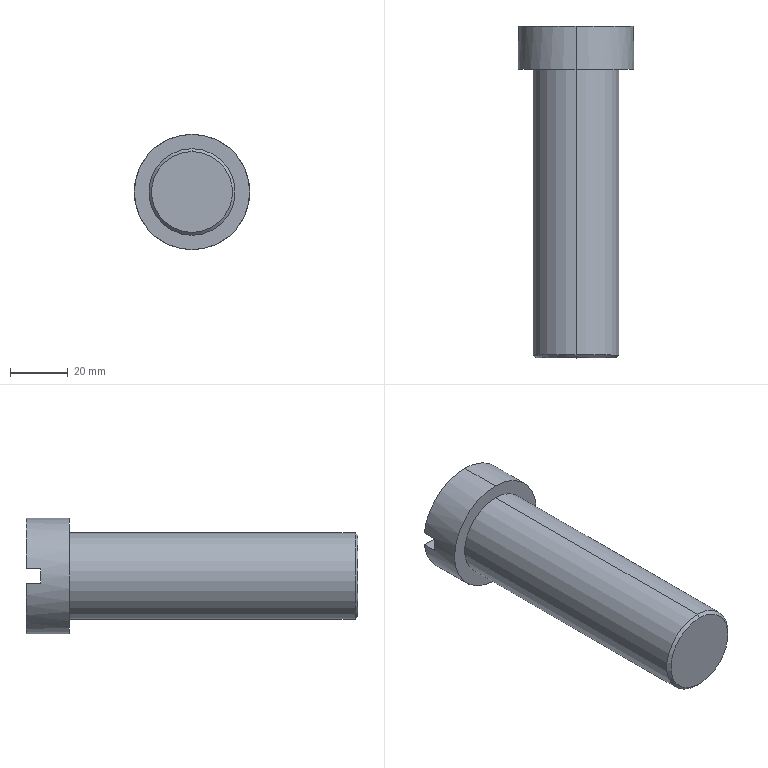Part | SolidWorks | features ICE 2, Chamfer 1, Extrusion 1 | 1 solid | 13 faces | box 40 x 115 x 40 mm | volume 88492 mm3 | plane 7 | cylinder 4 | cone 2 | commonest cylinder face diameters 30 x2 40 x2
STEP:
#1=CARTESIAN_POINT('',(0.,-50.,-14.));
#2=VERTEX_POINT('',#1);
#3=CARTESIAN_POINT('',(0.,-50.,14.));
#4=VERTEX_POINT('',#3);
#5=CARTESIAN_POINT('',(0.,-50.,0.));
#6=DIRECTION('',(0.,-1.,0.));
#7=DIRECTION('',(0.,0.,1.));
#8=AXIS2_PLACEMENT_3D('',#5,#6,#7);
#9=CIRCLE('',#8,14.);
#10=EDGE_CURVE('',#2,#4,#9,.T.);
#11=ORIENTED_EDGE('',*,*,#10,.F.);
#12=CARTESIAN_POINT('',(0.,-49.,-15.));
#13=VERTEX_POINT('',#12);
#14=CARTESIAN_POINT('',(0.,-49.,-15.));
#15=DIRECTION('',(0.,0.7071,-0.7071));
#16=VECTOR('',#15,1000.);
#17=LINE('',#14,#16);
#18=EDGE_CURVE('',#2,#13,#17,.T.);
#19=ORIENTED_EDGE('',*,*,#18,.T.);
#20=CARTESIAN_POINT('',(0.,-49.,15.));
#21=VERTEX_POINT('',#20);
#22=CARTESIAN_POINT('',(0.,-49.,0.));
#23=DIRECTION('',(0.,1.,0.));
#24=DIRECTION('',(0.,0.,1.));
#25=AXIS2_PLACEMENT_3D('',#22,#23,#24);
#26=CIRCLE('',#25,15.);
#27=EDGE_CURVE('',#21,#13,#26,.T.);
#28=ORIENTED_EDGE('',*,*,#27,.F.);
#29=CARTESIAN_POINT('',(0.,-49.,15.));
#30=DIRECTION('',(0.,0.7071,0.7071));
#31=VECTOR('',#30,1000.);
#32=LINE('',#29,#31);
#33=EDGE_CURVE('',#4,#21,#32,.T.);
#34=ORIENTED_EDGE('',*,*,#33,.F.);
#35=EDGE_LOOP('',(#11,#19,#28,#34));
#36=FACE_OUTER_BOUND('',#35,.T.);
#37=CARTESIAN_POINT('',(0.,-49.,0.));
#38=DIRECTION('',(0.,1.,0.));
#39=DIRECTION('',(0.,0.,1.));
#40=AXIS2_PLACEMENT_3D('',#37,#38,#39);
#41=CONICAL_SURFACE('',#40,15.,0.7854);
#42=ADVANCED_FACE('',(#36),#41,.T.);
#43=CARTESIAN_POINT('',(0.,50.,15.));
#44=VERTEX_POINT('',#43);
#45=CARTESIAN_POINT('',(0.,50.,-15.));
#46=VERTEX_POINT('',#45);
#47=CARTESIAN_POINT('',(0.,50.,0.));
#48=DIRECTION('',(0.,1.,0.));
#49=DIRECTION('',(0.,0.,1.));
#50=AXIS2_PLACEMENT_3D('',#47,#48,#49);
#51=CIRCLE('',#50,15.);
#52=EDGE_CURVE('',#44,#46,#51,.T.);
#53=ORIENTED_EDGE('',*,*,#52,.F.);
#54=CARTESIAN_POINT('',(0.,50.,15.));
#55=DIRECTION('',(0.,-1.,0.));
#56=VECTOR('',#55,1000.);
#57=LINE('',#54,#56);
#58=EDGE_CURVE('',#44,#21,#57,.T.);
#59=ORIENTED_EDGE('',*,*,#58,.T.);
#60=ORIENTED_EDGE('',*,*,#27,.T.);
#61=CARTESIAN_POINT('',(0.,50.,-15.));
#62=DIRECTION('',(0.,-1.,0.));
#63=VECTOR('',#62,1000.);
#64=LINE('',#61,#63);
#65=EDGE_CURVE('',#46,#13,#64,.T.);
#66=ORIENTED_EDGE('',*,*,#65,.F.);
#67=EDGE_LOOP('',(#53,#59,#60,#66));
#68=FACE_OUTER_BOUND('',#67,.T.);
#69=CARTESIAN_POINT('',(0.,50.,0.));
#70=DIRECTION('',(0.,-1.,0.));
#71=DIRECTION('',(0.,0.,-1.));
#72=AXIS2_PLACEMENT_3D('',#69,#70,#71);
#73=CYLINDRICAL_SURFACE('',#72,15.);
#74=ADVANCED_FACE('',(#68),#73,.T.);
#75=CARTESIAN_POINT('',(0.,65.,20.));
#76=VERTEX_POINT('',#75);
#77=CARTESIAN_POINT('',(19.843,65.,2.5));
#78=VERTEX_POINT('',#77);
#79=CARTESIAN_POINT('',(0.,65.,0.));
#80=DIRECTION('',(0.,1.,0.));
#81=DIRECTION('',(0.,0.,1.));
#82=AXIS2_PLACEMENT_3D('',#79,#80,#81);
#83=CIRCLE('',#82,20.);
#84=EDGE_CURVE('',#76,#78,#83,.T.);
#85=ORIENTED_EDGE('',*,*,#84,.F.);
#86=CARTESIAN_POINT('',(0.,50.,20.));
#87=VERTEX_POINT('',#86);
#88=CARTESIAN_POINT('',(0.,65.,20.));
#89=DIRECTION('',(0.,-1.,0.));
#90=VECTOR('',#89,1000.);
#91=LINE('',#88,#90);
#92=EDGE_CURVE('',#76,#87,#91,.T.);
#93=ORIENTED_EDGE('',*,*,#92,.T.);
#94=CARTESIAN_POINT('',(0.,50.,-20.));
#95=VERTEX_POINT('',#94);
#96=CARTESIAN_POINT('',(0.,50.,0.));
#97=DIRECTION('',(0.,1.,0.));
#98=DIRECTION('',(0.,0.,1.));
#99=AXIS2_PLACEMENT_3D('',#96,#97,#98);
#100=CIRCLE('',#99,20.);
#101=EDGE_CURVE('',#87,#95,#100,.T.);
#102=ORIENTED_EDGE('',*,*,#101,.T.);
#103=CARTESIAN_POINT('',(0.,65.,-20.));
#104=VERTEX_POINT('',#103);
#105=CARTESIAN_POINT('',(0.,65.,-20.));
#106=DIRECTION('',(0.,-1.,0.));
#107=VECTOR('',#106,1000.);
#108=LINE('',#105,#107);
#109=EDGE_CURVE('',#104,#95,#108,.T.);
#110=ORIENTED_EDGE('',*,*,#109,.F.);
#111=CARTESIAN_POINT('',(19.843,65.,-2.5));
#112=VERTEX_POINT('',#111);
#113=CARTESIAN_POINT('',(0.,65.,0.));
#114=DIRECTION('',(0.,1.,0.));
#115=DIRECTION('',(0.,0.,1.));
#116=AXIS2_PLACEMENT_3D('',#113,#114,#115);
#117=CIRCLE('',#116,20.);
#118=EDGE_CURVE('',#112,#104,#117,.T.);
#119=ORIENTED_EDGE('',*,*,#118,.F.);
#120=CARTESIAN_POINT('',(19.843,60.,-2.5));
#121=VERTEX_POINT('',#120);
#122=CARTESIAN_POINT('',(19.843,65.,-2.5));
#123=DIRECTION('',(0.,1.,0.));
#124=VECTOR('',#123,1000.);
#125=LINE('',#122,#124);
#126=EDGE_CURVE('',#121,#112,#125,.T.);
#127=ORIENTED_EDGE('',*,*,#126,.F.);
#128=CARTESIAN_POINT('',(19.843,60.,2.5));
#129=VERTEX_POINT('',#128);
#130=CARTESIAN_POINT('',(0.,60.,0.));
#131=DIRECTION('',(0.,-1.,0.));
#132=DIRECTION('',(0.,0.,-1.));
#133=AXIS2_PLACEMENT_3D('',#130,#131,#132);
#134=CIRCLE('',#133,20.);
#135=EDGE_CURVE('',#121,#129,#134,.T.);
#136=ORIENTED_EDGE('',*,*,#135,.T.);
#137=CARTESIAN_POINT('',(19.843,65.,2.5));
#138=DIRECTION('',(0.,1.,0.));
#139=VECTOR('',#138,1000.);
#140=LINE('',#137,#139);
#141=EDGE_CURVE('',#129,#78,#140,.T.);
#142=ORIENTED_EDGE('',*,*,#141,.T.);
#143=EDGE_LOOP('',(#85,#93,#102,#110,#119,#127,#136,#142));
#144=FACE_OUTER_BOUND('',#143,.T.);
#145=CARTESIAN_POINT('',(0.,65.,0.));
#146=DIRECTION('',(0.,-1.,0.));
#147=DIRECTION('',(0.,0.,-1.));
#148=AXIS2_PLACEMENT_3D('',#145,#146,#147);
#149=CYLINDRICAL_SURFACE('',#148,20.);
#150=ADVANCED_FACE('',(#144),#149,.T.);
#151=ORIENTED_EDGE('',*,*,#92,.F.);
#152=CARTESIAN_POINT('',(-19.843,65.,2.5));
#153=VERTEX_POINT('',#152);
#154=CARTESIAN_POINT('',(0.,65.,0.));
#155=DIRECTION('',(0.,1.,0.));
#156=DIRECTION('',(0.,0.,1.));
#157=AXIS2_PLACEMENT_3D('',#154,#155,#156);
#158=CIRCLE('',#157,20.);
#159=EDGE_CURVE('',#153,#76,#158,.T.);
#160=ORIENTED_EDGE('',*,*,#159,.F.);
#161=CARTESIAN_POINT('',(-19.843,60.,2.5));
#162=VERTEX_POINT('',#161);
#163=CARTESIAN_POINT('',(-19.843,65.,2.5));
#164=DIRECTION('',(0.,-1.,0.));
#165=VECTOR('',#164,1000.);
#166=LINE('',#163,#165);
#167=EDGE_CURVE('',#153,#162,#166,.T.);
#168=ORIENTED_EDGE('',*,*,#167,.T.);
#169=CARTESIAN_POINT('',(-19.843,60.,-2.5));
#170=VERTEX_POINT('',#169);
#171=CARTESIAN_POINT('',(0.,60.,0.));
#172=DIRECTION('',(0.,-1.,0.));
#173=DIRECTION('',(0.,0.,-1.));
#174=AXIS2_PLACEMENT_3D('',#171,#172,#173);
#175=CIRCLE('',#174,20.);
#176=EDGE_CURVE('',#162,#170,#175,.T.);
#177=ORIENTED_EDGE('',*,*,#176,.T.);
#178=CARTESIAN_POINT('',(-19.843,65.,-2.5));
#179=VERTEX_POINT('',#178);
#180=CARTESIAN_POINT('',(-19.843,65.,-2.5));
#181=DIRECTION('',(0.,-1.,0.));
#182=VECTOR('',#181,1000.);
#183=LINE('',#180,#182);
#184=EDGE_CURVE('',#179,#170,#183,.T.);
#185=ORIENTED_EDGE('',*,*,#184,.F.);
#186=CARTESIAN_POINT('',(0.,65.,0.));
#187=DIRECTION('',(0.,1.,0.));
#188=DIRECTION('',(0.,0.,1.));
#189=AXIS2_PLACEMENT_3D('',#186,#187,#188);
#190=CIRCLE('',#189,20.);
#191=EDGE_CURVE('',#104,#179,#190,.T.);
#192=ORIENTED_EDGE('',*,*,#191,.F.);
#193=ORIENTED_EDGE('',*,*,#109,.T.);
#194=CARTESIAN_POINT('',(0.,50.,0.));
#195=DIRECTION('',(0.,1.,0.));
#196=DIRECTION('',(0.,0.,1.));
#197=AXIS2_PLACEMENT_3D('',#194,#195,#196);
#198=CIRCLE('',#197,20.);
#199=EDGE_CURVE('',#95,#87,#198,.T.);
#200=ORIENTED_EDGE('',*,*,#199,.T.);
#201=EDGE_LOOP('',(#151,#160,#168,#177,#185,#192,#193,#200));
#202=FACE_OUTER_BOUND('',#201,.T.);
#203=CARTESIAN_POINT('',(0.,65.,0.));
#204=DIRECTION('',(0.,-1.,0.));
#205=DIRECTION('',(0.,0.,-1.));
#206=AXIS2_PLACEMENT_3D('',#203,#204,#205);
#207=CYLINDRICAL_SURFACE('',#206,20.);
#208=ADVANCED_FACE('',(#202),#207,.T.);
#209=ORIENTED_EDGE('',*,*,#118,.T.);
#210=ORIENTED_EDGE('',*,*,#191,.T.);
#211=CARTESIAN_POINT('',(0.,65.,-2.5));
#212=DIRECTION('',(1.,0.,0.));
#213=VECTOR('',#212,1000.);
#214=LINE('',#211,#213);
#215=EDGE_CURVE('',#179,#112,#214,.T.);
#216=ORIENTED_EDGE('',*,*,#215,.T.);
#217=EDGE_LOOP('',(#209,#210,#216));
#218=FACE_OUTER_BOUND('',#217,.T.);
#219=CARTESIAN_POINT('',(0.,65.,0.));
#220=DIRECTION('',(0.,1.,0.));
#221=DIRECTION('',(0.,0.,1.));
#222=AXIS2_PLACEMENT_3D('',#219,#220,#221);
#223=PLANE('',#222);
#224=ADVANCED_FACE('',(#218),#223,.T.);
#225=ORIENTED_EDGE('',*,*,#58,.F.);
#226=CARTESIAN_POINT('',(0.,50.,0.));
#227=DIRECTION('',(0.,1.,0.));
#228=DIRECTION('',(0.,0.,1.));
#229=AXIS2_PLACEMENT_3D('',#226,#227,#228);
#230=CIRCLE('',#229,15.);
#231=EDGE_CURVE('',#46,#44,#230,.T.);
#232=ORIENTED_EDGE('',*,*,#231,.F.);
#233=ORIENTED_EDGE('',*,*,#65,.T.);
#234=CARTESIAN_POINT('',(0.,-49.,0.));
#235=DIRECTION('',(0.,1.,0.));
#236=DIRECTION('',(0.,0.,1.));
#237=AXIS2_PLACEMENT_3D('',#234,#235,#236);
#238=CIRCLE('',#237,15.);
#239=EDGE_CURVE('',#13,#21,#238,.T.);
#240=ORIENTED_EDGE('',*,*,#239,.T.);
#241=EDGE_LOOP('',(#225,#232,#233,#240));
#242=FACE_OUTER_BOUND('',#241,.T.);
#243=CARTESIAN_POINT('',(0.,50.,0.));
#244=DIRECTION('',(0.,-1.,0.));
#245=DIRECTION('',(0.,0.,-1.));
#246=AXIS2_PLACEMENT_3D('',#243,#244,#245);
#247=CYLINDRICAL_SURFACE('',#246,15.);
#248=ADVANCED_FACE('',(#242),#247,.T.);
#249=CARTESIAN_POINT('',(0.,-50.,0.));
#250=DIRECTION('',(0.,-1.,0.));
#251=DIRECTION('',(0.,0.,1.));
#252=AXIS2_PLACEMENT_3D('',#249,#250,#251);
#253=CIRCLE('',#252,14.);
#254=EDGE_CURVE('',#4,#2,#253,.T.);
#255=ORIENTED_EDGE('',*,*,#254,.T.);
#256=ORIENTED_EDGE('',*,*,#10,.T.);
#257=EDGE_LOOP('',(#255,#256));
#258=FACE_OUTER_BOUND('',#257,.T.);
#259=CARTESIAN_POINT('',(0.,-50.,0.));
#260=DIRECTION('',(0.,1.,0.));
#261=DIRECTION('',(0.,0.,1.));
#262=AXIS2_PLACEMENT_3D('',#259,#260,#261);
#263=PLANE('',#262);
#264=ADVANCED_FACE('',(#258),#263,.F.);
#265=CARTESIAN_POINT('',(0.,65.,2.5));
#266=DIRECTION('',(1.,0.,0.));
#267=VECTOR('',#266,1000.);
#268=LINE('',#265,#267);
#269=EDGE_CURVE('',#153,#78,#268,.T.);
#270=ORIENTED_EDGE('',*,*,#269,.F.);
#271=ORIENTED_EDGE('',*,*,#159,.T.);
#272=ORIENTED_EDGE('',*,*,#84,.T.);
#273=EDGE_LOOP('',(#270,#271,#272));
#274=FACE_OUTER_BOUND('',#273,.T.);
#275=CARTESIAN_POINT('',(0.,65.,0.));
#276=DIRECTION('',(0.,1.,0.));
#277=DIRECTION('',(0.,0.,1.));
#278=AXIS2_PLACEMENT_3D('',#275,#276,#277);
#279=PLANE('',#278);
#280=ADVANCED_FACE('',(#274),#279,.T.);
#281=ORIENTED_EDGE('',*,*,#231,.T.);
#282=ORIENTED_EDGE('',*,*,#52,.T.);
#283=EDGE_LOOP('',(#281,#282));
#284=FACE_BOUND('',#283,.T.);
#285=ORIENTED_EDGE('',*,*,#199,.F.);
#286=ORIENTED_EDGE('',*,*,#101,.F.);
#287=EDGE_LOOP('',(#285,#286));
#288=FACE_OUTER_BOUND('',#287,.T.);
#289=CARTESIAN_POINT('',(0.,50.,0.));
#290=DIRECTION('',(0.,1.,0.));
#291=DIRECTION('',(0.,0.,1.));
#292=AXIS2_PLACEMENT_3D('',#289,#290,#291);
#293=PLANE('',#292);
#294=ADVANCED_FACE('',(#284,#288),#293,.F.);
#295=CARTESIAN_POINT('',(-30.092,60.,-2.5));
#296=DIRECTION('',(1.,0.,0.));
#297=VECTOR('',#296,1000.);
#298=LINE('',#295,#297);
#299=EDGE_CURVE('',#170,#121,#298,.T.);
#300=ORIENTED_EDGE('',*,*,#299,.F.);
#301=ORIENTED_EDGE('',*,*,#176,.F.);
#302=CARTESIAN_POINT('',(-30.092,60.,2.5));
#303=DIRECTION('',(1.,0.,0.));
#304=VECTOR('',#303,1000.);
#305=LINE('',#302,#304);
#306=EDGE_CURVE('',#162,#129,#305,.T.);
#307=ORIENTED_EDGE('',*,*,#306,.T.);
#308=ORIENTED_EDGE('',*,*,#135,.F.);
#309=EDGE_LOOP('',(#300,#301,#307,#308));
#310=FACE_OUTER_BOUND('',#309,.T.);
#311=CARTESIAN_POINT('',(0.,60.,0.));
#312=DIRECTION('',(0.,-1.,0.));
#313=DIRECTION('',(0.,0.,-1.));
#314=AXIS2_PLACEMENT_3D('',#311,#312,#313);
#315=PLANE('',#314);
#316=ADVANCED_FACE('',(#310),#315,.F.);
#317=ORIENTED_EDGE('',*,*,#184,.T.);
#318=ORIENTED_EDGE('',*,*,#299,.T.);
#319=ORIENTED_EDGE('',*,*,#126,.T.);
#320=ORIENTED_EDGE('',*,*,#215,.F.);
#321=EDGE_LOOP('',(#317,#318,#319,#320));
#322=FACE_OUTER_BOUND('',#321,.T.);
#323=CARTESIAN_POINT('',(-30.092,60.,-2.5));
#324=DIRECTION('',(0.,0.,1.));
#325=DIRECTION('',(1.,0.,0.));
#326=AXIS2_PLACEMENT_3D('',#323,#324,#325);
#327=PLANE('',#326);
#328=ADVANCED_FACE('',(#322),#327,.T.);
#329=ORIENTED_EDGE('',*,*,#269,.T.);
#330=ORIENTED_EDGE('',*,*,#141,.F.);
#331=ORIENTED_EDGE('',*,*,#306,.F.);
#332=ORIENTED_EDGE('',*,*,#167,.F.);
#333=EDGE_LOOP('',(#329,#330,#331,#332));
#334=FACE_OUTER_BOUND('',#333,.T.);
#335=CARTESIAN_POINT('',(-30.092,60.,2.5));
#336=DIRECTION('',(0.,0.,1.));
#337=DIRECTION('',(1.,0.,0.));
#338=AXIS2_PLACEMENT_3D('',#335,#336,#337);
#339=PLANE('',#338);
#340=ADVANCED_FACE('',(#334),#339,.F.);
#341=ORIENTED_EDGE('',*,*,#18,.F.);
#342=ORIENTED_EDGE('',*,*,#254,.F.);
#343=ORIENTED_EDGE('',*,*,#33,.T.);
#344=ORIENTED_EDGE('',*,*,#239,.F.);
#345=EDGE_LOOP('',(#341,#342,#343,#344));
#346=FACE_OUTER_BOUND('',#345,.T.);
#347=CARTESIAN_POINT('',(0.,-49.,0.));
#348=DIRECTION('',(0.,1.,0.));
#349=DIRECTION('',(0.,0.,1.));
#350=AXIS2_PLACEMENT_3D('',#347,#348,#349);
#351=CONICAL_SURFACE('',#350,15.,0.7854);
#352=ADVANCED_FACE('',(#346),#351,.T.);
#353=CLOSED_SHELL('',(#42,#74,#150,#208,#224,#248,#264,#280,#294,#316,#328,#340,#352));
#354=MANIFOLD_SOLID_BREP('',#353);
#355=CARTESIAN_POINT('',(0.,0.,0.));
#356=DIRECTION('',(0.,0.,1.));
#357=DIRECTION('',(1.,0.,0.));
#358=AXIS2_PLACEMENT_3D('',#355,#356,#357);
#359=(LENGTH_UNIT()NAMED_UNIT(*)SI_UNIT(.MILLI.,.METRE.));
#360=UNCERTAINTY_MEASURE_WITH_UNIT(LENGTH_MEASURE(0.00001),#359,'','');
#361=(NAMED_UNIT(*)PLANE_ANGLE_UNIT()SI_UNIT($,.RADIAN.));
#362=(NAMED_UNIT(*)SI_UNIT($,.STERADIAN.)SOLID_ANGLE_UNIT());
#363=(GEOMETRIC_REPRESENTATION_CONTEXT(3)GLOBAL_UNCERTAINTY_ASSIGNED_CONTEXT((#360))GLOBAL_UNIT_ASSIGNED_CONTEXT((#359,#361,#362))REPRESENTATION_CONTEXT('',''));
#364=ADVANCED_BREP_SHAPE_REPRESENTATION('',(#354,#358),#363);